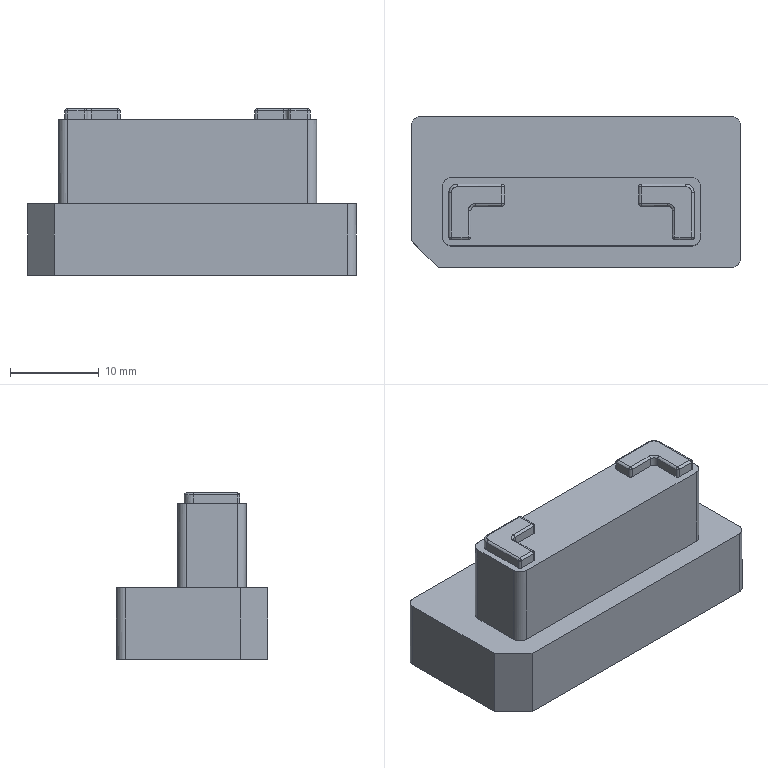NC program | PowerMill | posted with a generic post | part box 37 x 17 x 18.689 mm
Lines 4372 to 5650 of 30982:
N4469 M6
N4470 S8500 M03
N4471 G00 G90 X0.0 Y0.0
N4472 G43 Z11.799 H3
N4473
N4474 G05 P10000 R8
N4475 X24.2981 Y3.8845
N4476 Z-0.2719
N4477 G01 Z-1.4719 F360.0
N4478 X19.2336 Y2.4091 F600.0
N4479 X18.1581
N4480 X18.2134 Y2.2799
N4481 X18.325 Y1.9813
N4482 X18.4077 Y1.7309
N4483 X18.5015 Y1.3826
N4484 X18.5563 Y1.1401
N4485 X18.613 Y0.8096
N4486 X18.6467 Y0.5479
N4487 X18.6676 Y0.2849
N4488 X18.6776 Y0.0844
N4489 X18.6815 Y-0.1163
N4490 Y-2.2507
N4491 X19.4971 Y-2.2506
N4492 X19.497 Y0.6356
N4493 X19.4816 Y1.03
N4494 X19.4545 Y1.3278
N4495 X19.4178 Y1.5988
N4496 X19.3587 Y1.9199
N4497 X19.2826 Y2.241
N4498 X19.1948 Y2.5422
N4499 X19.103 Y2.8111
N4500 X19.0247 Y3.0129
N4501 X18.941 Y3.2126
N4502 X18.8309 Y3.4478
N4503 X18.7082 Y3.6817
N4504 X18.5791 Y3.9121
N4505 X18.4181 Y4.1676
N4506 X18.1622 Y4.5263
N4507 X17.9367 Y4.8049
N4508 X17.7727 Y4.987
N4509 X17.6035 Y5.1643
N4510 X17.2935 Y5.4558
N4511 X16.9722 Y5.7203
N4512 X16.6578 Y5.9462
N4513 X16.4356 Y6.0922
N4514 X16.3302 Y6.1561
N4515 X16.0141 Y6.3326
N4516 G03 X14.9435 Y6.7738 I-3.0645 J-5.9157
N4517 G01 X14.7245 Y6.8382
N4518 X14.3886 Y6.9201
N4519 X14.0825 Y6.979
N4520 X13.786 Y7.0208
N4521 X13.5247 Y7.0469
N4522 X13.1201 Y7.0663
N4523 X-14.0685 Y7.067
N4524 X-14.2967 Y7.0599
N4525 X-14.5247 Y7.0469
N4526 X-14.7728 Y7.0228
N4527 X-15.0349 Y6.9864
N4528 X-15.3679 Y6.9246
N4529 X-15.6723 Y6.8523
N4530 X-16.0708 Y6.7332
N4531 X-16.3195 Y6.6443
N4532 X-16.6494 Y6.5082
N4533 X-16.853 Y6.4136
N4534 X-17.0685 Y6.3017
N4535 X-17.2815 Y6.185
N4536 X-17.4712 Y6.0699
N4537 X-17.6561 Y5.9473
N4538 X-17.9255 Y5.7559
N4539 X-18.2215 Y5.5169
N4540 X-18.3911 Y5.3668
N4541 X-18.6473 Y5.1205
N4542 X-18.9368 Y4.8047
N4543 X-19.2086 Y4.4652
N4544 X-19.4183 Y4.1675
N4545 G03 X-19.7585 Y3.5872 I4.9244 J-3.2765
N4546 G01 X-19.8358 Y3.4381
N4547 X-19.9408 Y3.2132
N4548 X-20.0245 Y3.0132
N4549 X-20.1028 Y2.8111
N4550 X-20.1957 Y2.5391
N4551 X-20.2343 Y2.4068
N4552 X-19.1599 Y2.4069
N4553 X-19.2708 Y2.1312
N4554 X-19.325 Y1.9813
N4555 X-19.4077 Y1.7309
N4556 X-19.478 Y1.4766
N4557 G03 X-19.5947 Y0.9295 I5.7915 J-1.5213
N4558 G01 X-19.6298 Y0.692
N4559 X-19.6543 Y0.4532
N4560 G03 X-19.6811 Y-0.0516 I6.2831 J-0.5867
N4561 G01 X-19.6813 Y-2.2529
N4562 X-20.4971
N4563 X-20.4972 Y-5.0606
N4564 X-20.4903 Y-5.3578
N4565 X-20.4759 Y-5.6113
N4566 G03 X-20.3492 Y-6.4681 I6.8412 J0.5744
N4567 G01 X-20.3028 Y-6.6659
N4568 X-20.2341 Y-6.9127
N4569 X-19.3799
N4570 X-19.3234 Y-7.0729
N4571 X-19.2438 Y-7.2744
N4572 X-19.1512 Y-7.4833
N4573 X-19.0315 Y-7.7257
N4574 X-18.8997 Y-7.9617
N4575 X-18.7246 Y-8.2387
N4576 X-18.6037 Y-8.4137
N4577 X-18.4761 Y-8.5838
N4578 X-18.3418 Y-8.7487
N4579 X-18.1357 Y-8.9791
N4580 X-17.9571 Y-9.1603
N4581 X-17.7859 Y-9.3189
N4582 X-17.6044 Y-9.4746
N4583 X-17.4396 Y-9.6044
N4584 X-17.2341 Y-9.7531
N4585 X-17.0339 Y-9.8845
N4586 X-16.8461 Y-9.9981
N4587 X-16.6539 Y-10.1041
N4588 X-16.4336 Y-10.2139
N4589 X-16.2816 Y-10.283
N4590 X-16.1276 Y-10.3473
N4591 X-15.8989 Y-10.4336
N4592 X-15.6818 Y-10.5047
N4593 G03 X-15.1001 Y-10.6508 I1.6389 J5.2945
N4594 G01 X-14.8095 Y-10.6996
N4595 X-14.5553 Y-10.7298
N4596 X-14.2839 Y-10.7486
N4597 X-14.0173 Y-10.7553
N4598 X-12.1077
N4599 X-11.8253 Y-10.7478
N4600 X-11.4844 Y-10.7194
N4601 X-11.2528 Y-10.6898
N4602 X-11.0227 Y-10.6503
N4603 X-10.7945 Y-10.6008
N4604 X-10.5687 Y-10.5415
N4605 X-10.2854 Y-10.4523
N4606 X-10.054 Y-10.3692
N4607 X-9.8266 Y-10.2755
N4608 X-9.6037 Y-10.1716
N4609 X-9.3858 Y-10.0576
N4610 X-9.117 Y-9.8992
N4611 X-8.9049 Y-9.762
N4612 X-8.6995 Y-9.615
N4613 X-8.5011 Y-9.4585
N4614 X-8.3104 Y-9.2929
N4615 X-8.0802 Y-9.0711
N4616 X-7.9058 Y-8.8884
N4617 X-7.7402 Y-8.6976
N4618 X-7.5837 Y-8.4993
N4619 X-7.4368 Y-8.2938
N4620 X-7.265 Y-8.0254
N4621 X-7.1411 Y-7.8129
N4622 X-7.0271 Y-7.595
N4623 X-6.9232 Y-7.3722
N4624 X-6.8296 Y-7.1448
N4625 X-6.7609 Y-6.9614
N4626 X-6.7349 Y-6.9119
N4627 X5.733 Y-6.9112
N4628 G00 Z5.7323
N4629 G01 X13.9681 Y6.0315 F10000.0
N4630 G00 Z-1.3719
N4631 G01 X14.0735 Y6.0033 Z-1.3738 F360.0
N4632 X14.3646 Y5.9102 Z-1.3791
N4633 X14.652 Y5.8065 Z-1.3845
N4634 X14.8808 Y5.7108 Z-1.3888
N4635 X15.1729 Y5.571 Z-1.3944
N4636 X15.4593 Y5.42 Z-1.4001
N4637 X15.6806 Y5.2883 Z-1.4046
N4638 X15.9394 Y5.1157 Z-1.41
N4639 X16.1918 Y4.9339 Z-1.4154
N4640 X16.366 Y4.7957 Z-1.4193
N4641 X16.7519 Y4.4499 Z-1.4284
N4642 X17.0023 Y4.1918 Z-1.4346
N4643 X17.2378 Y3.9199 Z-1.4409
N4644 X17.4575 Y3.6352 Z-1.4472
N4645 X17.6006 Y3.4321 Z-1.4515
N4646 X17.7353 Y3.2233 Z-1.4559
N4647 X17.9271 Y2.8882 Z-1.4626
N4648 X18.0993 Y2.5426 Z-1.4693
N4649 X18.126 Y2.4838 Z-1.4705
N4650 X18.1581 Y2.4091 Z-1.4719
N4651 X18.2134 Y2.2799 F600.0
N4652 X18.325 Y1.9813
N4653 X18.4077 Y1.7309
N4654 X18.5015 Y1.3826
N4655 X18.5563 Y1.1401
N4656 X18.613 Y0.8096
N4657 X18.6467 Y0.5479
N4658 X18.6676 Y0.2849
N4659 X18.6776 Y0.0844
N4660 X18.6815 Y-0.1163
N4661 Y-5.091
N4662 X18.6741 Y-5.3734
N4663 X18.6456 Y-5.7143
N4664 X18.6161 Y-5.946
N4665 X18.5766 Y-6.1761
N4666 X18.5271 Y-6.4043
N4667 X18.4677 Y-6.6301
N4668 X18.3786 Y-6.9134
N4669 X18.2954 Y-7.1448
N4670 X18.2018 Y-7.3722
N4671 X18.0979 Y-7.595
N4672 X17.9839 Y-7.8129
N4673 X17.8254 Y-8.0817
N4674 X17.6882 Y-8.2938
N4675 X17.5413 Y-8.4993
N4676 X17.3848 Y-8.6976
N4677 X17.2192 Y-8.8884
N4678 X16.9974 Y-9.1185
N4679 X16.8146 Y-9.2929
N4680 X16.6239 Y-9.4585
N4681 X16.4255 Y-9.615
N4682 X16.2201 Y-9.762
N4683 X15.9516 Y-9.9338
N4684 X15.7392 Y-10.0576
N4685 X15.5213 Y-10.1716
N4686 X15.2984 Y-10.2755
N4687 X15.071 Y-10.3692
N4688 X14.8396 Y-10.4523
N4689 X14.5563 Y-10.5415
N4690 X14.3305 Y-10.6008
N4691 X14.1023 Y-10.6503
N4692 X13.8722 Y-10.6898
N4693 X13.5813 Y-10.7256
N4694 X13.2997 Y-10.7478
N4695 X13.0173 Y-10.7553
N4696 X11.1077
N4697 X10.8099 Y-10.7471
N4698 X10.5697 Y-10.7298
N4699 X10.3155 Y-10.6996
N4700 X10.0249 Y-10.6508
N4701 G02 X8.9141 Y-10.3132 I1.0903 J5.5839
N4702 G01 X8.6914 Y-10.2139
N4703 X8.4711 Y-10.1041
N4704 X8.2789 Y-9.9981
N4705 X8.0911 Y-9.8845
N4706 X7.8909 Y-9.7531
N4707 X7.6854 Y-9.6044
N4708 X7.5206 Y-9.4746
N4709 X7.3391 Y-9.3189
N4710 X7.1679 Y-9.1603
N4711 X6.9893 Y-8.9791
N4712 X6.7832 Y-8.7487
N4713 X6.6489 Y-8.5838
N4714 X6.5213 Y-8.4137
N4715 X6.3844 Y-8.2145
N4716 X6.2546 Y-8.0106
N4717 X6.1477 Y-7.826
N4718 X6.0482 Y-7.6374
N4719 X5.9434 Y-7.4166
N4720 X5.8556 Y-7.212
N4721 X5.775 Y-6.9996
N4722 G03 X5.4169 Y-6.6477 I-0.561 J-0.2128
N4723 G01 X5.2852 Y-6.6004
N4724 X5.0578 Y-6.5068
N4725 X4.835 Y-6.4029
N4726 X4.6171 Y-6.2889
N4727 X4.3483 Y-6.1304
N4728 X4.1362 Y-5.9932
N4729 X3.9307 Y-5.8463
N4730 X3.7324 Y-5.6898
N4731 X3.5416 Y-5.5242
N4732 X3.3115 Y-5.3024
N4733 X3.1371 Y-5.1196
N4734 X2.9715 Y-4.9289
N4735 X2.815 Y-4.7305
N4736 X2.668 Y-4.5251
N4737 X2.4962 Y-4.2566
N4738 X2.3724 Y-4.0442
N4739 X2.2584 Y-3.8263
N4740 X2.1545 Y-3.6034
N4741 X2.0608 Y-3.376
N4742 X1.9777 Y-3.1446
N4743 X1.8885 Y-2.8613
N4744 X1.8292 Y-2.6355
N4745 X1.7797 Y-2.4073
N4746 X1.7402 Y-2.1772
N4747 X1.7044 Y-1.8863
N4748 X1.6822 Y-1.6047
N4749 X1.6747 Y-1.3223
N4750 Y0.5872
N4751 X1.6829 Y0.8851
N4752 X1.7002 Y1.1253
N4753 X1.7304 Y1.3795
N4754 X1.7792 Y1.6701
N4755 G02 X2.1168 Y2.7809 I5.5839 J-1.0903
N4756 G01 X2.2161 Y3.0036
N4757 X2.3259 Y3.2239
N4758 X2.4319 Y3.4161
N4759 X2.5455 Y3.6039
N4760 X2.6769 Y3.8041
N4761 X2.8256 Y4.0096
N4762 X2.9554 Y4.1744
N4763 X3.1111 Y4.3559
N4764 X3.2697 Y4.5271
N4765 X3.4509 Y4.7057
N4766 X3.6813 Y4.9118
N4767 X3.8462 Y5.0461
N4768 X4.0163 Y5.1737
N4769 X4.2155 Y5.3106
N4770 X4.4194 Y5.4404
N4771 X4.604 Y5.5473
N4772 X4.7926 Y5.6468
N4773 X5.0134 Y5.7516
N4774 X5.218 Y5.8394
N4775 X5.4402 Y5.9237
N4776 G02 X6.0294 Y6.0972 I1.8315 J-5.1332
N4777 G01 X6.263 Y6.1482
N4778 X6.4987 Y6.1888
N4779 X6.7669 Y6.2221
N4780 X6.9792 Y6.24
N4781 X7.206 Y6.2499
N4782 X12.3138 Y6.2515
N4783 X12.5553 Y6.2459
N4784 X12.7966 Y6.2314
N4785 X13.0297 Y6.2109
N4786 X13.2617 Y6.1803
N4787 G02 X13.8474 Y6.0638 I-1.3349 J-8.2417
N4788 G01 X14.0735 Y6.0033
N4789 G02 X14.652 Y5.8065 I-2.3699 J-7.9159
N4790 G01 X14.8808 Y5.7108
N4791 G02 X15.4593 Y5.42 I-3.4838 J-7.6506
N4792 G01 X15.6806 Y5.2883
N4793 G02 X16.1918 Y4.9339 I-4.6202 J-7.2098
N4794 G01 X16.366 Y4.7957
N4795 X16.5617 Y4.6259
N4796 X16.7519 Y4.4499
N4797 G02 X17.4575 Y3.6352 I-4.4479 J-4.5655
N4798 G02 X17.7353 Y3.2233 I-4.9274 J-3.6225
N4799 G02 X18.0993 Y2.5426 I-5.74 J-3.5074
N4800 G01 X18.1581 Y2.4091
N4801 G00 Z5.7305
N4802 G01 X-19.6814 Y-3.2522 F10000.0
N4803 G00 Z-1.3719
N4804 G01 X-19.6811 Y-0.0516 Z-1.4277 F360.0
N4805 X-19.6728 Y0.2011 Z-1.4321
N4806 X-19.6543 Y0.4532 Z-1.4366
N4807 X-19.6298 Y0.692 Z-1.4407
N4808 X-19.5947 Y0.9295 Z-1.4449
N4809 X-19.5427 Y1.2044 Z-1.4498
N4810 X-19.478 Y1.4766 Z-1.4547
N4811 X-19.4077 Y1.7309 Z-1.4593
N4812 X-19.325 Y1.9813 Z-1.4639
N4813 X-19.2134 Y2.2799 Z-1.4695
N4814 X-19.1599 Y2.4069 Z-1.4719
N4815 X-19.0812 Y2.5818 F600.0
N4816 X-18.9976 Y2.7545
N4817 X-18.8704 Y2.9911
N4818 X-18.7353 Y3.2233
N4819 G02 X-18.0911 Y4.092 I5.4223 J-3.348
N4820 G01 X-17.9251 Y4.2744
N4821 X-17.7519 Y4.4499
N4822 G02 X-17.1918 Y4.9339 I4.6842 J-4.8551
N4823 G02 X-16.6806 Y5.2883 I5.1314 J-6.8554
N4824 G01 X-16.4593 Y5.42
N4825 G02 X-15.8808 Y5.7108 I4.0623 J-7.3598
N4826 G01 X-15.652 Y5.8065
N4827 G02 X-15.0735 Y6.0033 I2.9484 J-7.7191
N4828 G01 X-14.8474 Y6.0638
N4829 G02 X-14.2617 Y6.1803 I1.9206 J-8.1252
N4830 G01 X-14.0297 Y6.2109
N4831 X-13.7605 Y6.2339
N4832 X-13.4908 Y6.2486
N4833 X-13.3138 Y6.2515
N4834 X-8.339
N4835 X-8.0566 Y6.2441
N4836 X-7.7157 Y6.2156
N4837 X-7.484 Y6.1861
N4838 X-7.2539 Y6.1466
N4839 X-7.0258 Y6.0971
N4840 X-6.7999 Y6.0377
N4841 X-6.5166 Y5.9486
N4842 X-6.2852 Y5.8654
N4843 X-6.0578 Y5.7718
N4844 X-5.835 Y5.6679
N4845 X-5.6171 Y5.5539
N4846 X-5.3483 Y5.3954
N4847 X-5.1362 Y5.2582
N4848 X-4.9307 Y5.1113
N4849 X-4.7324 Y4.9548
N4850 X-4.5416 Y4.7892
N4851 X-4.3115 Y4.5674
N4852 X-4.1371 Y4.3846
N4853 X-3.9715 Y4.1939
N4854 X-3.815 Y3.9955
N4855 X-3.668 Y3.7901
N4856 X-3.4962 Y3.5216
N4857 X-3.3724 Y3.3092
N4858 X-3.2584 Y3.0913
N4859 X-3.1545 Y2.8684
N4860 X-3.0608 Y2.641
N4861 X-2.9777 Y2.4096
N4862 X-2.8885 Y2.1263
N4863 X-2.8292 Y1.9005
N4864 X-2.7797 Y1.6723
N4865 X-2.7402 Y1.4422
N4866 X-2.7044 Y1.1513
N4867 X-2.6822 Y0.8697
N4868 X-2.6747 Y0.5872
N4869 Y-1.3223
N4870 X-2.6829 Y-1.6202
N4871 X-2.7002 Y-1.8603
N4872 X-2.7304 Y-2.1145
N4873 X-2.7792 Y-2.4051
N4874 G02 X-3.1168 Y-3.5159 I-5.5839 J1.0903
N4875 G01 X-3.2161 Y-3.7386
N4876 X-3.3259 Y-3.9589
N4877 X-3.4319 Y-4.1511
N4878 X-3.5455 Y-4.3389
N4879 X-3.6769 Y-4.5391
N4880 X-3.8256 Y-4.7446
N4881 X-3.9554 Y-4.9094
N4882 X-4.1111 Y-5.0909
N4883 X-4.2697 Y-5.2621
N4884 X-4.4509 Y-5.4407
N4885 X-4.6813 Y-5.6468
N4886 X-4.8462 Y-5.7811
N4887 X-5.0163 Y-5.9087
N4888 X-5.2155 Y-6.0456
N4889 X-5.4194 Y-6.1754
N4890 X-5.604 Y-6.2823
N4891 X-5.7926 Y-6.3818
N4892 X-6.0134 Y-6.4866
N4893 X-6.218 Y-6.5744
N4894 X-6.4304 Y-6.655
N4895 G03 X-6.7823 Y-7.0131 I0.2128 J-0.561
N4896 G01 X-6.8296 Y-7.1448
N4897 X-6.9232 Y-7.3722
N4898 X-7.0271 Y-7.595
N4899 X-7.1411 Y-7.8129
N4900 X-7.2996 Y-8.0817
N4901 X-7.4368 Y-8.2938
N4902 X-7.5837 Y-8.4993
N4903 X-7.7402 Y-8.6976
N4904 X-7.9058 Y-8.8884
N4905 X-8.1276 Y-9.1185
N4906 X-8.3104 Y-9.2929
N4907 X-8.5011 Y-9.4585
N4908 X-8.6995 Y-9.615
N4909 X-8.9049 Y-9.762
N4910 X-9.1734 Y-9.9338
N4911 X-9.3858 Y-10.0576
N4912 X-9.6037 Y-10.1716
N4913 X-9.8266 Y-10.2755
N4914 X-10.054 Y-10.3692
N4915 X-10.2854 Y-10.4523
N4916 X-10.5687 Y-10.5415
N4917 X-10.7945 Y-10.6008
N4918 X-11.0227 Y-10.6503
N4919 X-11.2528 Y-10.6898
N4920 X-11.5437 Y-10.7256
N4921 X-11.8253 Y-10.7478
N4922 X-12.1077 Y-10.7553
N4923 X-14.0173
N4924 X-14.3151 Y-10.7471
N4925 X-14.5553 Y-10.7298
N4926 X-14.8095 Y-10.6996
N4927 X-15.1001 Y-10.6508
N4928 G02 X-15.6818 Y-10.5047 I1.0572 J5.4406
N4929 G01 X-15.8989 Y-10.4336
N4930 X-16.1276 Y-10.3473
N4931 X-16.2816 Y-10.283
N4932 X-16.4336 Y-10.2139
N4933 X-16.6539 Y-10.1041
N4934 X-16.8461 Y-9.9981
N4935 X-17.0339 Y-9.8845
N4936 X-17.2341 Y-9.7531
N4937 X-17.4396 Y-9.6044
N4938 X-17.6044 Y-9.4746
N4939 X-17.7859 Y-9.3189
N4940 X-17.9571 Y-9.1603
N4941 X-18.1357 Y-8.9791
N4942 X-18.3418 Y-8.7487
N4943 X-18.4761 Y-8.5838
N4944 X-18.6037 Y-8.4137
N4945 X-18.7563 Y-8.1907
N4946 X-18.8997 Y-7.9617
N4947 X-19.0315 Y-7.7257
N4948 X-19.1512 Y-7.4833
N4949 X-19.2438 Y-7.2744
N4950 X-19.3234 Y-7.0729
N4951 X-19.3932 Y-6.8751
N4952 X-19.4552 Y-6.6748
N4953 X-19.5217 Y-6.4224
N4954 X-19.5795 Y-6.1601
N4955 X-19.6241 Y-5.8953
N4956 X-19.6586 Y-5.5946
N4957 X-19.6735 Y-5.3907
N4958 X-19.6815 Y-5.091
N4959 X-19.6811 Y-0.0516
N4960 G02 X-19.6543 Y0.4532 I6.3099 J-0.0819
N4961 G01 X-19.6298 Y0.692
N4962 X-19.5947 Y0.9295
N4963 G02 X-19.478 Y1.4766 I5.9082 J-0.9742
N4964 G01 X-19.4077 Y1.7309
N4965 X-19.325 Y1.9813
N4966 X-19.2134 Y2.2799
N4967 X-19.1599 Y2.4069
N4968 G00 Z3.9991
N4969 G01 X1.3433 Y5.3856 F10000.0
N4970 G00 Z0.9291
N4971 G01 Z-0.2709 F360.0
N4972 X-3.3785 Y3.0339 F600.0
N4973 X-19.3993 Y1.2381
N4974 X-19.4547 Y0.9632
N4975 X-19.5024 Y0.6425
N4976 X-19.5352 Y0.3203
N4977 X-19.5486 Y-0.0017
N4978 X-19.5376 Y-0.6332
N4979 Y-3.0154
N4980 X-2.8108 Y-1.1404
N4981 X-2.8061 Y-1.2663
N4982 X-2.8117 Y-1.5884
N4983 X-2.8367 Y-1.9103
N4984 X-2.8807 Y-2.2324
N4985 X-2.9444 Y-2.5541
N4986 X-3.0277 Y-2.8763
N4987 X-3.133 Y-3.1984
N4988 X-3.2613 Y-3.5202
N4989 X-3.4134 Y-3.8423
N4990 X-3.5924 Y-4.164
N4991 X-3.8001 Y-4.4862
N4992 X-4.0381 Y-4.8023
N4993 X-4.1784 Y-4.9678
N4994 X-4.3237 Y-5.1288
N4995 X-4.5165 Y-5.3229
N4996 X-4.6555 Y-5.4506
N4997 X-4.8376 Y-5.6056
N4998 X-19.126 Y-7.2072
N4999 G00 Z3.9991
N5000 G01 X5.3639 Y11.212 F10000.0
N5001 G00 Z0.9291
N5002 G01 Z-0.2709 F360.0
N5003 X6.3534 Y6.0307 F600.0
N5004 X5.6812 Y-6.5986
N5005 X5.794 Y-6.6345
N5006 X5.9125 Y-6.9924
N5007 X6.042 Y-7.3147
N5008 X6.1972 Y-7.6365
N5009 X6.3976 Y-7.9921
N5010 X6.5875 Y-8.2787
N5011 X6.7187 Y-8.4587
N5012 X6.8321 Y-8.6015
N5013 X7.0405 Y-8.8411
N5014 X7.1182 Y-8.9235
N5015 X7.3629 Y-9.163
N5016 X7.4549 Y-9.2449
N5017 X7.6814 Y-9.4343
N5018 X7.8407 Y-9.5555
N5019 X8.0087 Y-9.6737
N5020 X8.3532 Y-9.8887
N5021 X8.6528 Y-10.0487
N5022 X9.0104 Y-10.21
N5023 X9.2963 Y-10.3197
N5024 X9.6183 Y-10.4209
N5025 X9.7418 Y-10.4516
N5026 X10.6232 Y6.1075
N5027 X11.8538 Y6.1071
N5028 X12.1714 Y6.1179
N5029 X12.4933 Y6.1183
N5030 X12.8146 Y6.1003
N5031 X13.1364 Y6.0653
N5032 X13.4569 Y6.012
N5033 X13.7781 Y5.9438
N5034 X14.0995 Y5.8578
N5035 X14.4212 Y5.7527
N5036 X14.7421 Y5.6264
N5037 X14.8604 Y5.5728
N5038 X14.0031 Y-10.5351
N5039 G00 Z11.799
N5040 G05 P0
N5041 (---------------)
N5042 ( END TOOLPATH : 精公基准台01-平坦面平行-D10 )
N5043 (---------------)
N5044 ( START TOOLPATH : 精公基准台01-基准面偏置-D10 )
N5045 (---------------)
N5046 G00 X0.0 Y0.0 Z9.7991
N5047 G05 P10000 R8
N5048 X26.3922 Y15.1849
N5049 Z-9.69
N5050 G01 Z-10.89 F360.0
N5051 X22.3865 Y11.7527 F600.0
N5052 X12.6724 Y6.9672
N5053 X13.2063 Y6.964
N5054 X13.4873 Y6.95
N5055 X13.7683 Y6.9231
N5056 X14.0493 Y6.8831
N5057 X14.3303 Y6.8309
N5058 X14.6112 Y6.7649
N5059 X14.8922 Y6.6857
N5060 X15.1289 Y6.6077
N5061 X15.4542 Y6.4837
N5062 X15.7352 Y6.3596
N5063 X16.0162 Y6.2186
N5064 X16.2436 Y6.0914
N5065 X16.4728 Y5.9502
N5066 X16.5781 Y5.8802
N5067 X16.8591 Y5.6808
N5068 X17.1401 Y5.456
N5069 X17.2246 Y5.3835
N5070 X17.4614 Y5.1647
N5071 X17.7021 Y4.9184
N5072 X17.794 Y4.8168
N5073 X18.0304 Y4.5335
N5074 X18.2641 Y4.2172
N5075 X18.4403 Y3.9481
N5076 X18.5955 Y3.6834
N5077 X18.7165 Y3.4538
N5078 X18.826 Y3.2261
N5079 X18.8743 Y3.1168
N5080 X18.9886 Y2.8334
N5081 X19.0881 Y2.5501
N5082 X19.1726 Y2.2667
N5083 X19.2428 Y1.9834
N5084 X19.2998 Y1.7001
N5085 X19.3433 Y1.4167
N5086 X19.3721 Y1.1543
N5087 X19.3916 Y0.85
N5088 X19.3973 Y0.2833
N5089 Y-4.8168
N5090 X19.3894 Y-5.3835
N5091 X19.3709 Y-5.6729
N5092 X19.3391 Y-5.9502
N5093 X19.2939 Y-6.2335
N5094 X19.236 Y-6.5169
N5095 X19.1641 Y-6.8002
N5096 X19.0782 Y-7.0836
N5097 X18.9775 Y-7.3669
N5098 X18.826 Y-7.7299
N5099 X18.7095 Y-7.9723
N5100 X18.5791 Y-8.2169
N5101 X18.4298 Y-8.469
N5102 X18.2201 Y-8.7836
N5103 X18.0071 Y-9.0669
N5104 X17.7674 Y-9.3503
N5105 X17.7021 Y-9.422
N5106 X17.4447 Y-9.6847
N5107 X17.1401 Y-9.9601
N5108 X16.8591 Y-10.1848
N5109 X16.5781 Y-10.3849
N5110 X16.4264 Y-10.4837
N5111 X16.2213 Y-10.6081
N5112 X16.0162 Y-10.7224
N5113 X15.7352 Y-10.8631
N5114 X15.4542 Y-10.9873
N5115 X15.2953 Y-11.0503
N5116 X14.8922 Y-11.1895
N5117 X14.6112 Y-11.2689
N5118 X14.3303 Y-11.3345
N5119 X14.0493 Y-11.3871
N5120 X13.7683 Y-11.4267
N5121 X13.4873 Y-11.4537
N5122 X13.2063 Y-11.4679
N5123 X12.6443 Y-11.4712
N5124 X-13.7683
N5125 X-14.3303 Y-11.4629
N5126 X-14.6112 Y-11.4433
N5127 X-14.8922 Y-11.4109
N5128 X-15.1732 Y-11.3654
N5129 X-15.4542 Y-11.3071
N5130 X-15.7352 Y-11.2354
N5131 X-16.0162 Y-11.15
N5132 X-16.2958 Y-11.0503
N5133 X-16.5781 Y-10.9347
N5134 X-16.8591 Y-10.8032
N5135 X-17.1401 Y-10.6544
N5136 X-17.4269 Y-10.4837
N5137 X-17.7021 Y-10.2994
N5138 X-17.9462 Y-10.1179
N5139 X-18.2641 Y-9.8522
N5140 X-18.5157 Y-9.6153
N5141 X-18.7673 Y-9.3503
N5142 X-19.0334 Y-9.0337
N5143 X-19.2201 Y-8.7836
N5144 X-19.388 Y-8.5346
N5145 X-19.579 Y-8.2169
N5146 X-19.729 Y-7.9336
N5147 X-19.8616 Y-7.6502
N5148 X-19.95 Y-7.4375
N5149 X-20.0784 Y-7.0836
N5150 X-20.1642 Y-6.8002
N5151 X-20.2359 Y-6.5169
N5152 X-20.2942 Y-6.2335
N5153 X-20.3393 Y-5.9502
N5154 X-20.3712 Y-5.6668
N5155 X-20.3904 Y-5.3835
N5156 X-20.3975 Y-4.8168
N5157 Y0.2833
N5158 X-20.3917 Y0.85
N5159 X-20.374 Y1.1334
N5160 X-20.3432 Y1.4167
N5161 X-20.2996 Y1.7001
N5162 X-20.2427 Y1.9834
N5163 X-20.1724 Y2.2667
N5164 X-20.088 Y2.5501
N5165 X-19.95 Y2.9339
N5166 X-19.8745 Y3.1168
N5167 X-19.7438 Y3.4001
N5168 X-19.5954 Y3.6834
N5169 X-19.388 Y4.0307
N5170 X-19.2412 Y4.2501
N5171 X-19.0449 Y4.5152
N5172 X-18.7939 Y4.8168
N5173 X-18.5444 Y5.0827
N5174 X-18.2245 Y5.3835
N5175 X-17.9633 Y5.6006
N5176 X-17.7021 Y5.7958
N5177 X-17.473 Y5.9502
N5178 X-17.1401 Y6.1508
N5179 X-16.8591 Y6.2994
N5180 X-16.5781 Y6.4308
N5181 X-16.3718 Y6.5169
N5182 X-16.0162 Y6.6461
N5183 X-15.7352 Y6.7316
N5184 X-15.4542 Y6.8035
N5185 X-15.1732 Y6.8618
N5186 X-14.8922 Y6.907
N5187 X-14.6112 Y6.9396
N5188 X-14.3303 Y6.9596
N5189 X-13.7683 Y6.9673
N5190 X12.6724 Y6.9672
N5191 G00 Z9.7991
N5192 G05 P0
N5193 (---------------)
N5194 ( END TOOLPATH : 精公基准台01-基准面偏置-D10 )
N5195 (---------------)
N5196 ( START TOOLPATH : 精公基准台01-外形侧光-D10 )
N5197 (---------------)
N5198 G00 X0.0 Y0.0 Z10.799
N5199 G05 P10000 R8
N5200 X17.2611 Y-10.0609
N5201 Z-9.66
N5202 G01 Z-10.86 F360.0
N5203 G03 X16.1261 Y-10.2338 I-0.3588 J-1.4564 F600.0
N5204 G02 X12.9615 Y-11.101 I-3.1109 J5.1446
N5205 G01 X-0.5477 Y-11.1009
N5206 X-14.0589 Y-11.1008
N5207 G02 X-20.0272 Y-5.1116 I0.0425 J6.0107
N5208 G01 Y0.5486
N5209 G02 X-14.0568 Y6.5971 I6.0109 J0.0376
N5210 G01 X12.9622 Y6.5973
N5211 G02 X19.0273 Y0.5477 I0.053 J-6.012
N5212 G01 X19.0272 Y-5.1134
N5213 G02 X16.1261 Y-10.2338 I-6.012 J0.0242
N5214 G03 X15.4458 Y-11.1586 I0.7762 J-1.2835
N5215 G01 X17.1763 Y-10.0293
N5216 G03 X16.0399 Y-10.1922 I-0.3716 J-1.4533
N5217 G02 X12.9615 Y-11.021 I-3.0247 J5.103
N5218 G01 X-0.5477 Y-11.0209
N5219 X-14.0568 Y-11.0208
N5220 G02 X-19.9472 Y-5.1116 I0.0404 J5.9307
N5221 G01 X-19.9473 Y0.5477
N5222 G02 X-14.0568 Y6.5171 I5.9309 J0.0385
N5223 G01 X12.9615 Y6.5173
N5224 G02 X18.9473 Y0.5477 I0.0537 J-5.9319
N5225 G01 X18.9472 Y-5.1116
N5226 G02 X16.0399 Y-10.1922 I-5.932 J0.0224
N5227 G03 X15.3514 Y-11.1109 I0.7648 J-1.2904
N5228 G00 Z10.799
N5229 G05 P0
N5230 (---------------)
N5231 ( END TOOLPATH : 精公基准台01-外形侧光-D10 )
N5232 (---------------)
N5233 ( START TOOLPATH : 精公基准台01-基准台侧光-D10 )
N5234 (---------------)
N5235 G00 X0.0 Y0.0 Z9.7991
N5236 G05 P10000 R8
N5237 X23.8104 Y-16.6059
N5238 Z-17.59
N5239 G01 Z-18.79 F360.0
N5240 G03 X20.9346 Y-12.5157 I-1.4379 J2.0451 F600.0
N5241 G01 X20.9116 Y-12.5318
N5242 X20.9102 Y-12.5328
N5243 X20.9088 Y-12.5337
N5244 X20.6286 Y-12.7132
N5245 X20.6264 Y-12.7145
N5246 X20.6242 Y-12.7158
N5247 X20.2721 Y-12.9111
N5248 X20.2701 Y-12.9121
N5249 X20.2681 Y-12.9131
N5250 X20.0181 Y-13.034
N5251 X20.016 Y-13.035
N5252 X20.0139 Y-13.0359
N5253 X19.6316 Y-13.194
N5254 X19.6293 Y-13.1949
N5255 X19.6269 Y-13.1958
N5256 X19.3108 Y-13.304
N5257 X19.3092 Y-13.3045
N5258 X19.3076 Y-13.305
N5259 X19.139 Y-13.3548
N5260 X19.1379 Y-13.3551
N5261 X19.1369 Y-13.3554
N5262 X18.9893 Y-13.3946
N5263 X18.9878 Y-13.395
N5264 X18.9862 Y-13.3954
N5265 X18.6701 Y-13.4662
N5266 X18.668 Y-13.4666
N5267 X18.6659 Y-13.467
N5268 X18.3497 Y-13.5203
N5269 X18.3476 Y-13.5206
N5270 X18.3455 Y-13.5209
N5271 X18.0293 Y-13.5567
N5272 X18.0272 Y-13.557
N5273 X18.025 Y-13.5571
N5274 X17.7089 Y-13.5757
N5275 X17.707 Y-13.5758
N5276 X17.7052
N5277 X17.3891 Y-13.58
N5278 X17.3885
N5279 X17.388
N5280 X-15.4911
N5281 X-15.4923
N5282 X-15.4935
N5283 X-15.8097 Y-13.5705
N5284 X-15.8122 Y-13.5704
N5285 X-15.8147 Y-13.5702
N5286 X-16.1309 Y-13.5406
N5287 X-16.1334 Y-13.5404
N5288 X-16.1359 Y-13.54
N5289 X-16.4521 Y-13.49
N5290 X-16.4546 Y-13.4895
N5291 X-16.4571 Y-13.489
N5292 X-16.7733 Y-13.4178
N5293 X-16.7758 Y-13.4172
N5294 X-16.7784 Y-13.4165
N5295 X-17.0945 Y-13.3232
N5296 X-17.097 Y-13.3224
N5297 X-17.0996 Y-13.3216
N5298 X-17.4157 Y-13.2049
N5299 X-17.4183 Y-13.2039
N5300 X-17.4208 Y-13.2028
N5301 X-17.7369 Y-13.0609
N5302 X-17.7395 Y-13.0597
N5303 X-17.742 Y-13.0584
N5304 X-18.0581 Y-12.8888
N5305 X-18.0605 Y-12.8875
N5306 X-18.0628 Y-12.8861
N5307 X-18.3376 Y-12.7136
N5308 X-18.3402 Y-12.7119
N5309 X-18.3427 Y-12.7101
N5310 X-18.7002 Y-12.4452
N5311 X-18.7019 Y-12.4439
N5312 X-18.7035 Y-12.4426
N5313 X-18.7655 Y-12.3914
N5314 X-18.7668 Y-12.3903
N5315 X-18.7681 Y-12.3892
N5316 X-19.0222 Y-12.1606
N5317 X-19.0236 Y-12.1593
N5318 X-19.0249 Y-12.1581
N5319 X-19.1137 Y-12.0705
N5320 X-19.1139 Y-12.0703
N5321 X-19.1141 Y-12.0701
N5322 X-21.9594 Y-9.2248
N5323 X-21.9596 Y-9.2246
N5324 X-21.9597 Y-9.2245
N5325 X-22.1871 Y-8.9945
N5326 X-22.188 Y-8.9936
N5327 X-22.1889 Y-8.9926
N5328 X-22.2687 Y-8.9064
N5329 X-22.27 Y-8.905
N5330 X-22.2712 Y-8.9035
N5331 X-22.5076 Y-8.6217
N5332 X-22.5096 Y-8.6192
N5333 X-22.5115 Y-8.6166
N5334 X-22.7608 Y-8.2662
N5335 X-22.762 Y-8.2643
N5336 X-22.7632 Y-8.2625
N5337 X-22.8302 Y-8.1563
N5338 X-22.8309 Y-8.1551
N5339 X-22.8317 Y-8.1538
N5340 X-22.9536 Y-7.9438
N5341 X-22.9547 Y-7.9417
N5342 X-22.9558 Y-7.9396
N5343 X-23.1149 Y-7.6234
N5344 X-23.1161 Y-7.6209
N5345 X-23.1172 Y-7.6184
N5346 X-23.2495 Y-7.3022
N5347 X-23.2505 Y-7.2997
N5348 X-23.2514 Y-7.2972
N5349 X-23.3593 Y-6.981
N5350 X-23.3601 Y-6.9785
N5351 X-23.3608 Y-6.976
N5352 X-23.4458 Y-6.6598
N5353 X-23.4464 Y-6.6573
N5354 X-23.447 Y-6.6548
N5355 X-23.5103 Y-6.3386
N5356 X-23.5107 Y-6.3361
N5357 X-23.5111 Y-6.3336
N5358 X-23.5536 Y-6.0174
N5359 X-23.5539 Y-6.0149
N5360 X-23.5541 Y-6.0123
N5361 X-23.5762 Y-5.6962
N5362 X-23.5763 Y-5.6939
N5363 X-23.5764 Y-5.6915
N5364 X-23.58 Y-5.3754
N5365 Y-5.3749
N5366 Y-5.3745
N5367 X-23.5792 Y7.5875
N5368 Y7.5891
N5369 Y7.5907
N5370 X-23.5663 Y7.9069
N5371 X-23.5662 Y7.909
N5372 X-23.5661 Y7.9111
N5373 X-23.5363 Y8.2273
N5374 X-23.536 Y8.2294
N5375 X-23.5357 Y8.2315
N5376 X-23.489 Y8.5476
N5377 X-23.4887 Y8.5498
N5378 X-23.4883 Y8.5519
N5379 X-23.424 Y8.868
N5380 X-23.4236 Y8.8701
N5381 X-23.4231 Y8.8722
N5382 X-23.3407 Y9.1884
N5383 X-23.3402 Y9.1905
N5384 X-23.3395 Y9.1926
N5385 X-23.2384 Y9.5087
N5386 X-23.2377 Y9.5108
N5387 X-23.2369 Y9.5129
N5388 X-23.1162 Y9.8291
N5389 X-23.1153 Y9.8312
N5390 X-23.1144 Y9.8333
N5391 X-22.9721 Y10.1495
N5392 X-22.9712 Y10.1514
N5393 X-22.9703 Y10.1534
N5394 X-22.8336 Y10.4181
N5395 X-22.8324 Y10.4202
N5396 X-22.8313 Y10.4223
N5397 X-22.6128 Y10.7898
N5398 X-22.6118 Y10.7915
N5399 X-22.6107 Y10.7932
N5400 X-22.513 Y10.9404
N5401 X-22.5123 Y10.9415
N5402 X-22.5115 Y10.9426
N5403 X-22.3911 Y11.1115
N5404 X-22.3899 Y11.1132
N5405 X-22.3887 Y11.1148
N5406 X-22.1383 Y11.4309
N5407 X-22.1366 Y11.433
N5408 X-22.1349 Y11.435
N5409 X-21.8733 Y11.7237
N5410 X-21.8715 Y11.7257
N5411 X-21.8695 Y11.7276
N5412 X-21.5534 Y12.0317
N5413 X-21.5513 Y12.0336
N5414 X-21.5491 Y12.0355
N5415 X-21.233 Y12.299
N5416 X-21.2315 Y12.3002
N5417 X-21.23 Y12.3014
N5418 X-21.1083 Y12.3935
N5419 X-21.1072 Y12.3943
N5420 X-21.1061 Y12.3951
N5421 X-20.9116 Y12.5318
N5422 X-20.9102 Y12.5328
N5423 X-20.9088 Y12.5337
N5424 X-20.6286 Y12.7132
N5425 X-20.6264 Y12.7145
N5426 X-20.6242 Y12.7158
N5427 X-20.2721 Y12.9111
N5428 X-20.2701 Y12.9121
N5429 X-20.2681 Y12.9131
N5430 X-20.0181 Y13.034
N5431 X-20.016 Y13.035
N5432 X-20.0139 Y13.0359
N5433 X-19.6316 Y13.194
N5434 X-19.6293 Y13.1949
N5435 X-19.6269 Y13.1958
N5436 X-19.3108 Y13.304
N5437 X-19.3087 Y13.3047
N5438 X-19.3066 Y13.3053
N5439 X-18.9904 Y13.3943
N5440 X-18.9883 Y13.3949
N5441 X-18.9862 Y13.3954
N5442 X-18.6701 Y13.4662
N5443 X-18.668 Y13.4666
N5444 X-18.6659 Y13.467
N5445 X-18.3497 Y13.5203
N5446 X-18.3476 Y13.5206
N5447 X-18.3455 Y13.5209
N5448 X-18.0293 Y13.5567
N5449 X-18.0272 Y13.557
N5450 X-18.025 Y13.5571
N5451 X-17.7089 Y13.5757
N5452 X-17.707 Y13.5758
N5453 X-17.7052
N5454 X-17.3891 Y13.58
N5455 X-17.3885
N5456 X-17.388
N5457 X0.0
N5458 X17.388
N5459 X17.3885
N5460 X17.389
N5461 X17.7052 Y13.576
N5462 X17.707 Y13.5759
N5463 X17.7089
N5464 X18.025 Y13.5573
N5465 X18.0272 Y13.5571
N5466 X18.0294 Y13.5569
N5467 X18.3455 Y13.5209
N5468 X18.3476 Y13.5206
N5469 X18.3497 Y13.5203
N5470 X18.6658 Y13.4672
N5471 X18.668 Y13.4668
N5472 X18.6701 Y13.4663
N5473 X18.9862 Y13.3954
N5474 X18.9883 Y13.3949
N5475 X18.9904 Y13.3944
N5476 X19.3066 Y13.3053
N5477 X19.3088 Y13.3047
N5478 X19.311 Y13.304
N5479 X19.6271 Y13.195
N5480 X19.6291 Y13.1943
N5481 X19.631 Y13.1935
N5482 X19.9472 Y13.0657
N5483 X19.9495 Y13.0648
N5484 X19.9517 Y13.0637
N5485 X20.2679 Y12.9124
N5486 X20.2698 Y12.9114
N5487 X20.2717 Y12.9104
N5488 X20.5879 Y12.7374
N5489 X20.5901 Y12.7361
N5490 X20.5923 Y12.7348
N5491 X20.9084 Y12.5347
N5492 X20.9101 Y12.5336
N5493 X20.9118 Y12.5325
N5494 X21.1062 Y12.395
N5495 X21.1073 Y12.3942
N5496 X21.1083 Y12.3935
N5497 X21.23 Y12.3014
N5498 X21.2314 Y12.3003
N5499 X21.2327 Y12.2993
N5500 X21.5041 Y12.0752
N5501 X21.5062 Y12.0735
N5502 X21.5082 Y12.0716
N5503 X21.8423 Y11.7555
N5504 X21.8445 Y11.7534
N5505 X21.8465 Y11.7512
N5506 X22.1341 Y11.4351
N5507 X22.1359 Y11.4331
N5508 X22.1376 Y11.431
N5509 X22.3886 Y11.1148
N5510 X22.3899 Y11.1131
N5511 X22.3912 Y11.1114
N5512 X22.5116 Y10.9417
N5513 X22.5123 Y10.9407
N5514 X22.5129 Y10.9397
N5515 X22.6105 Y10.7933
N5516 X22.6115 Y10.7918
N5517 X22.6124 Y10.7902
N5518 X22.8028 Y10.4741
N5519 X22.804 Y10.472
N5520 X22.8052 Y10.4698
N5521 X22.9703 Y10.1537
N5522 X22.9713 Y10.1516
N5523 X22.9723 Y10.1495
N5524 X23.1144 Y9.8333
N5525 X23.1153 Y9.8312
N5526 X23.1162 Y9.8291
N5527 X23.237 Y9.5129
N5528 X23.2378 Y9.5108
N5529 X23.2385 Y9.5087
N5530 X23.3396 Y9.1926
N5531 X23.3402 Y9.1905
N5532 X23.3408 Y9.1884
N5533 X23.4231 Y8.8722
N5534 X23.4236 Y8.8703
N5535 X23.424 Y8.8684
N5536 X23.4731 Y8.6335
N5537 X23.4735 Y8.6315
N5538 X23.4738 Y8.6295
N5539 X23.5357 Y8.2321
N5540 X23.536 Y8.2296
N5541 X23.5363 Y8.2271
N5542 X23.5653 Y7.911
N5543 X23.5655 Y7.909
N5544 X23.5656 Y7.9071
N5545 X23.5792 Y7.5909
N5546 Y7.5892
N5547 Y7.5875
N5548 Y-7.5875
N5549 Y-7.5891
N5550 Y-7.5907
N5551 X23.5664 Y-7.9069
N5552 X23.5662 Y-7.909
N5553 X23.5661 Y-7.9112
N5554 X23.5363 Y-8.2273
N5555 X23.536 Y-8.2294
N5556 X23.5357 Y-8.2315
N5557 X23.489 Y-8.5476
N5558 X23.4887 Y-8.5498
N5559 X23.4883 Y-8.5519
N5560 X23.424 Y-8.868
N5561 X23.4236 Y-8.8701
N5562 X23.4231 Y-8.8722
N5563 X23.3408 Y-9.1884
N5564 X23.3402 Y-9.1905
N5565 X23.3395 Y-9.1926
N5566 X23.2384 Y-9.5087
N5567 X23.2377 Y-9.5108
N5568 X23.2369 Y-9.5129
N5569 X23.1162 Y-9.8291
N5570 X23.1153 Y-9.8312
N5571 X23.1144 Y-9.8333
N5572 X22.9721 Y-10.1495
N5573 X22.9712 Y-10.1514
N5574 X22.9703 Y-10.1534
N5575 X22.8336 Y-10.4181
N5576 X22.8324 Y-10.4202
N5577 X22.8313 Y-10.4223
N5578 X22.6128 Y-10.7898
N5579 X22.6118 Y-10.7915
N5580 X22.6107 Y-10.7932
N5581 X22.513 Y-10.9404
N5582 X22.5123 Y-10.9415
N5583 X22.5115 Y-10.9426
N5584 X22.3911 Y-11.1115
N5585 X22.3899 Y-11.1132
N5586 X22.3887 Y-11.1148
N5587 X22.1383 Y-11.4309
N5588 X22.1366 Y-11.433
N5589 X22.1349 Y-11.435
N5590 X21.8733 Y-11.7237
N5591 X21.8715 Y-11.7257
N5592 X21.8695 Y-11.7276
N5593 X21.5534 Y-12.0317
N5594 X21.5513 Y-12.0336
N5595 X21.5491 Y-12.0355
N5596 X21.233 Y-12.299
N5597 X21.2315 Y-12.3002
N5598 X21.23 Y-12.3014
N5599 X21.1083 Y-12.3935
N5600 X21.1072 Y-12.3943
N5601 X21.1061 Y-12.3951
N5602 X20.9346 Y-12.5157
N5603 G03 X23.8104 Y-16.6059 I1.4379 J-2.0451
N5604 G01 X23.7584 Y-16.5446
N5605 G03 X20.8827 Y-12.4544 I-1.4379 J2.0451
N5606 G01 X20.8656 Y-12.4664
N5607 X20.5854 Y-12.6458
N5608 X20.2333 Y-12.8411
N5609 X19.9833 Y-12.962
N5610 X19.601 Y-13.1201
N5611 X19.2849 Y-13.2283
N5612 X19.1163 Y-13.2781
N5613 X18.9687 Y-13.3173
N5614 X18.6526 Y-13.3881
N5615 X18.3364 Y-13.4414
N5616 X18.0203 Y-13.4772
N5617 X17.7042 Y-13.4958
N5618 X17.388 Y-13.5
N5619 X-15.4911
N5620 X-15.8073 Y-13.4906
N5621 X-16.1234 Y-13.461
N5622 X-16.4396 Y-13.4109
N5623 X-16.7557 Y-13.3398
N5624 X-17.0719 Y-13.2465
N5625 X-17.388 Y-13.1299
N5626 X-17.7042 Y-12.988
N5627 X-18.0203 Y-12.8183
N5628 X-18.295 Y-12.6458
N5629 X-18.6526 Y-12.3809
N5630 X-18.7146 Y-12.3297
N5631 X-18.9687 Y-12.1011
N5632 X-19.0575 Y-12.0135
N5633 X-21.9028 Y-9.1682
N5634 X-22.1302 Y-8.9383
N5635 X-22.2099 Y-8.8521
N5636 X-22.4463 Y-8.5702
N5637 X-22.6956 Y-8.2198
N5638 X-22.7625 Y-8.1137
N5639 X-22.8844 Y-7.9036
N5640 X-23.0434 Y-7.5875
N5641 X-23.1757 Y-7.2714
N5642 X-23.2836 Y-6.9552
N5643 X-23.3685 Y-6.6391
N5644 X-23.4318 Y-6.3229
N5645 X-23.4743 Y-6.0068
N5646 X-23.4964 Y-5.6906
N5647 X-23.5 Y-5.3745
N5648 Y7.2714
N5649 X-23.4992 Y7.5875
N5650 X-23.4864 Y7.9036
N5651 X-23.4566 Y8.2198
N5652 X-23.4099 Y8.5359
N5653 X-23.3456 Y8.8521
N5654 X-23.2633 Y9.1682
N5655 X-23.1622 Y9.4844
N5656 X-23.0415 Y9.8005
N5657 X-22.8992 Y10.1167
N5658 X-22.7625 Y10.3814
N5659 X-22.544 Y10.749
N5660 X-22.4463 Y10.8961
N5661 X-22.3259 Y11.0651
N5662 X-22.0756 Y11.3812
N5663 X-21.8141 Y11.6699
N5664 X-21.4979 Y11.974
N5665 X-21.1818 Y12.2376
N5666 X-21.06 Y12.3297
N5667 X-20.8656 Y12.4664
N5668 X-20.5854 Y12.6458
N5669 X-20.2333 Y12.8411
N5670 X-19.9833 Y12.962
N5671 X-19.601 Y13.1201
N5672 X-19.2849 Y13.2283
N5673 X-18.9687 Y13.3173
N5674 X-18.6526 Y13.3881
N5675 X-18.3364 Y13.4414
N5676 X-18.0203 Y13.4772
N5677 X-17.7042 Y13.4958
N5678 X-17.388 Y13.5
N5679 X0.0
N5680 X17.388
N5681 X17.7042 Y13.496
N5682 X18.0203 Y13.4774
N5683 X18.3364 Y13.4414
N5684 X18.6526 Y13.3883
N5685 X18.9687 Y13.3174
N5686 X19.2849 Y13.2283
N5687 X19.601 Y13.1194
N5688 X19.9172 Y12.9916
N5689 X20.2333 Y12.8402
N5690 X20.5495 Y12.6672
N5691 X20.8656 Y12.4671
N5692 X21.06 Y12.3297
N5693 X21.1818 Y12.2376
N5694 X21.4532 Y12.0135
N5695 X21.7873 Y11.6974
N5696 X22.0749 Y11.3812
N5697 X22.3259 Y11.0651
N5698 X22.4463 Y10.8954
N5699 X22.5439 Y10.749
N5700 X22.7343 Y10.4328
N5701 X22.8993 Y10.1167
N5702 X23.0415 Y9.8005
N5703 X23.1623 Y9.4844
N5704 X23.2634 Y9.1682
N5705 X23.3457 Y8.8521
N5706 X23.3948 Y8.6172
N5707 X23.4566 Y8.2198
N5708 X23.4857 Y7.9036
N5709 X23.4992 Y7.5875
N5710 X23.5 Y7.2714
N5711 Y-6.9552
N5712 X23.4992 Y-7.5875
N5713 X23.4864 Y-7.9036
N5714 X23.4566 Y-8.2198
N5715 X23.4099 Y-8.5359
N5716 X23.3456 Y-8.8521
N5717 X23.2633 Y-9.1682
N5718 X23.1622 Y-9.4844
N5719 X23.0415 Y-9.8005
N5720 X22.8992 Y-10.1167
N5721 X22.7625 Y-10.3814
N5722 X22.544 Y-10.749
N5723 X22.4463 Y-10.8961
N5724 X22.3259 Y-11.0651
N5725 X22.0756 Y-11.3812
N5726 X21.8141 Y-11.6699
N5727 X21.4979 Y-11.974
N5728 X21.1818 Y-12.2376
N5729 X21.06 Y-12.3297
N5730 X20.8827 Y-12.4544
N5731 G03 X23.7584 Y-16.5446 I1.4378 J-2.0451
N5732 G00 Z9.7991
N5733 G05 P0
N5734 (---------------)
N5735 ( END TOOLPATH : 精公基准台01-基准台侧光-D10 )
N5736 (---------------)
N5737
N5738 M05
N5739 G53 Z0.0
N5740 (---------------)
N5741 ( START TOOLPATH : 精公精光01-等高-D3 )
N5742 (---------------)
N5743 ( TOOL NO.    :10 )
N5744 ( TOOL TYPE   : ENDMILL)
N5745 ( TOOL ID     : D3_1)
N5746 ( TOOL DIA    : 3.0 LENGTH 58.0)
N5747 T10